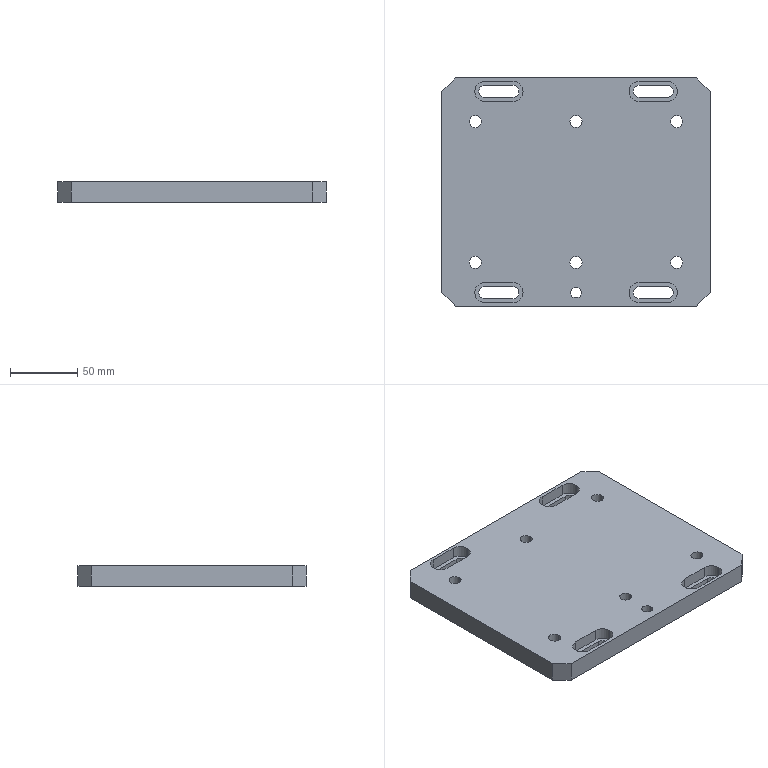Part | STEP file | 11-FGXW-07-0511 | 1 solid | 86 faces | box 200 x 170 x 15 mm | volume 471303 mm3 | cylinder 50 | plane 36 | commonest cylinder face diameters 9 x24 15 x24 8 x2